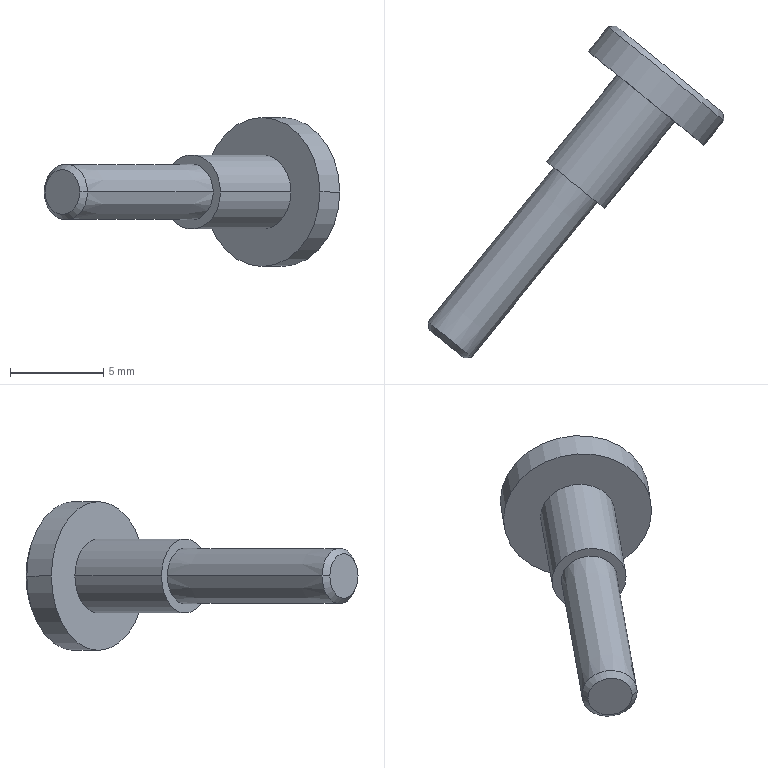Part | SolidWorks | features BaseBody 1 | 1 solid | 14 faces | box 15.875 x 17.831 x 8 mm | volume 252.086 mm3 | cone 6 | cylinder 4 | plane 4 | commonest cylinder face diameters 4 x2 8 x2
STEP:
#1=CARTESIAN_POINT('',(502.793,-146.387,330.545));
#2=VERTEX_POINT('',#1);
#3=CARTESIAN_POINT('',(505.117,-148.278,330.545));
#4=VERTEX_POINT('',#3);
#5=CARTESIAN_POINT('',(503.955,-147.333,330.545));
#6=DIRECTION('',(0.6309,0.7758,-0.000000012));
#7=DIRECTION('',(-0.4361,0.3546,-0.8271));
#8=AXIS2_PLACEMENT_3D('',#5,#6,#7);
#9=CIRCLE('',#8,1.498);
#10=EDGE_CURVE('',#2,#4,#9,.T.);
#11=ORIENTED_EDGE('',*,*,#10,.T.);
#12=CARTESIAN_POINT('',(511.87,-139.977,330.545));
#13=VERTEX_POINT('',#12);
#14=CARTESIAN_POINT('',(511.87,-139.977,330.545));
#15=DIRECTION('',(0.6311,0.7757,-0.000000012));
#16=VECTOR('',#15,1000.);
#17=LINE('',#14,#16);
#18=EDGE_CURVE('',#4,#13,#17,.T.);
#19=ORIENTED_EDGE('',*,*,#18,.T.);
#20=CARTESIAN_POINT('',(509.542,-138.085,330.545));
#21=VERTEX_POINT('',#20);
#22=CARTESIAN_POINT('',(510.706,-139.031,330.545));
#23=DIRECTION('',(-0.6309,-0.7758,0.000000012));
#24=DIRECTION('',(-0.7758,0.6309,0.));
#25=AXIS2_PLACEMENT_3D('',#22,#23,#24);
#26=CIRCLE('',#25,1.5);
#27=EDGE_CURVE('',#13,#21,#26,.T.);
#28=ORIENTED_EDGE('',*,*,#27,.T.);
#29=CARTESIAN_POINT('',(509.542,-138.085,330.545));
#30=DIRECTION('',(0.6308,0.7759,-0.000000012));
#31=VECTOR('',#30,1000.);
#32=LINE('',#29,#31);
#33=EDGE_CURVE('',#2,#21,#32,.T.);
#34=ORIENTED_EDGE('',*,*,#33,.F.);
#35=EDGE_LOOP('',(#11,#19,#28,#34));
#36=FACE_OUTER_BOUND('',#35,.T.);
#37=CARTESIAN_POINT('',(510.706,-139.031,330.545));
#38=DIRECTION('',(0.6309,0.7758,-0.000000012));
#39=DIRECTION('',(-0.7758,0.6309,0.));
#40=AXIS2_PLACEMENT_3D('',#37,#38,#39);
#41=CONICAL_SURFACE('',#40,1.5,0.0001745);
#42=ADVANCED_FACE('',(#36),#41,.T.);
#43=CARTESIAN_POINT('',(502.836,-146.809,330.545));
#44=VERTEX_POINT('',#43);
#45=CARTESIAN_POINT('',(504.695,-148.321,330.545));
#46=VERTEX_POINT('',#45);
#47=CARTESIAN_POINT('',(503.766,-147.565,330.545));
#48=DIRECTION('',(0.6309,0.7758,-0.000000012));
#49=DIRECTION('',(-0.7758,0.6309,0.));
#50=AXIS2_PLACEMENT_3D('',#47,#48,#49);
#51=CIRCLE('',#50,1.198);
#52=EDGE_CURVE('',#44,#46,#51,.T.);
#53=ORIENTED_EDGE('',*,*,#52,.T.);
#54=CARTESIAN_POINT('',(505.117,-148.278,330.545));
#55=DIRECTION('',(0.9947,0.1024,-0.000000009));
#56=VECTOR('',#55,1000.);
#57=LINE('',#54,#56);
#58=EDGE_CURVE('',#46,#4,#57,.T.);
#59=ORIENTED_EDGE('',*,*,#58,.T.);
#60=ORIENTED_EDGE('',*,*,#10,.F.);
#61=CARTESIAN_POINT('',(502.793,-146.387,330.545));
#62=DIRECTION('',(-0.1026,0.9947,-0.000000009));
#63=VECTOR('',#62,1000.);
#64=LINE('',#61,#63);
#65=EDGE_CURVE('',#44,#2,#64,.T.);
#66=ORIENTED_EDGE('',*,*,#65,.F.);
#67=EDGE_LOOP('',(#53,#59,#60,#66));
#68=FACE_OUTER_BOUND('',#67,.T.);
#69=CARTESIAN_POINT('',(503.955,-147.333,330.545));
#70=DIRECTION('',(0.6309,0.7758,-0.000000012));
#71=DIRECTION('',(-0.7758,0.6309,0.));
#72=AXIS2_PLACEMENT_3D('',#69,#70,#71);
#73=CONICAL_SURFACE('',#72,1.498,0.7855);
#74=ADVANCED_FACE('',(#68),#73,.T.);
#75=CARTESIAN_POINT('',(512.258,-140.293,330.545));
#76=VERTEX_POINT('',#75);
#77=CARTESIAN_POINT('',(509.154,-137.769,330.545));
#78=VERTEX_POINT('',#77);
#79=CARTESIAN_POINT('',(510.706,-139.031,330.545));
#80=DIRECTION('',(-0.6309,-0.7758,0.000000012));
#81=DIRECTION('',(-0.7758,0.6309,0.));
#82=AXIS2_PLACEMENT_3D('',#79,#80,#81);
#83=CIRCLE('',#82,2.);
#84=EDGE_CURVE('',#76,#78,#83,.T.);
#85=ORIENTED_EDGE('',*,*,#84,.F.);
#86=CARTESIAN_POINT('',(516.043,-135.638,330.545));
#87=VERTEX_POINT('',#86);
#88=CARTESIAN_POINT('',(516.043,-135.638,330.545));
#89=DIRECTION('',(0.6309,0.7758,-0.000000012));
#90=VECTOR('',#89,1000.);
#91=LINE('',#88,#90);
#92=EDGE_CURVE('',#76,#87,#91,.T.);
#93=ORIENTED_EDGE('',*,*,#92,.T.);
#94=CARTESIAN_POINT('',(512.94,-133.114,330.545));
#95=VERTEX_POINT('',#94);
#96=CARTESIAN_POINT('',(514.492,-134.376,330.545));
#97=DIRECTION('',(-0.6309,-0.7758,0.000000012));
#98=DIRECTION('',(-0.7758,0.6309,0.));
#99=AXIS2_PLACEMENT_3D('',#96,#97,#98);
#100=CIRCLE('',#99,2.);
#101=EDGE_CURVE('',#87,#95,#100,.T.);
#102=ORIENTED_EDGE('',*,*,#101,.T.);
#103=CARTESIAN_POINT('',(512.94,-133.114,330.545));
#104=DIRECTION('',(0.6309,0.7758,-0.000000012));
#105=VECTOR('',#104,1000.);
#106=LINE('',#103,#105);
#107=EDGE_CURVE('',#78,#95,#106,.T.);
#108=ORIENTED_EDGE('',*,*,#107,.F.);
#109=EDGE_LOOP('',(#85,#93,#102,#108));
#110=FACE_OUTER_BOUND('',#109,.T.);
#111=CARTESIAN_POINT('',(514.492,-134.376,330.545));
#112=DIRECTION('',(0.6309,0.7758,-0.000000012));
#113=DIRECTION('',(-0.7758,0.6309,0.));
#114=AXIS2_PLACEMENT_3D('',#111,#112,#113);
#115=CYLINDRICAL_SURFACE('',#114,2.);
#116=ADVANCED_FACE('',(#110),#115,.T.);
#117=CARTESIAN_POINT('',(517.595,-136.9,330.545));
#118=VERTEX_POINT('',#117);
#119=CARTESIAN_POINT('',(511.388,-131.852,330.545));
#120=VERTEX_POINT('',#119);
#121=CARTESIAN_POINT('',(514.492,-134.376,330.545));
#122=DIRECTION('',(-0.6309,-0.7758,0.000000012));
#123=DIRECTION('',(-0.7758,0.6309,0.));
#124=AXIS2_PLACEMENT_3D('',#121,#122,#123);
#125=CIRCLE('',#124,4.);
#126=EDGE_CURVE('',#118,#120,#125,.T.);
#127=ORIENTED_EDGE('',*,*,#126,.F.);
#128=CARTESIAN_POINT('',(518.668,-135.581,330.545));
#129=VERTEX_POINT('',#128);
#130=CARTESIAN_POINT('',(518.857,-135.348,330.545));
#131=DIRECTION('',(0.6309,0.7758,-0.000000012));
#132=VECTOR('',#131,1000.);
#133=LINE('',#130,#132);
#134=EDGE_CURVE('',#118,#129,#133,.T.);
#135=ORIENTED_EDGE('',*,*,#134,.T.);
#136=CARTESIAN_POINT('',(512.461,-130.533,330.545));
#137=VERTEX_POINT('',#136);
#138=CARTESIAN_POINT('',(515.564,-133.057,330.545));
#139=DIRECTION('',(-0.6309,-0.7758,0.000000012));
#140=DIRECTION('',(-0.7758,0.6309,0.));
#141=AXIS2_PLACEMENT_3D('',#138,#139,#140);
#142=CIRCLE('',#141,4.);
#143=EDGE_CURVE('',#129,#137,#142,.T.);
#144=ORIENTED_EDGE('',*,*,#143,.T.);
#145=CARTESIAN_POINT('',(512.65,-130.301,330.545));
#146=DIRECTION('',(0.6309,0.7758,-0.000000012));
#147=VECTOR('',#146,1000.);
#148=LINE('',#145,#147);
#149=EDGE_CURVE('',#120,#137,#148,.T.);
#150=ORIENTED_EDGE('',*,*,#149,.F.);
#151=EDGE_LOOP('',(#127,#135,#144,#150));
#152=FACE_OUTER_BOUND('',#151,.T.);
#153=CARTESIAN_POINT('',(515.753,-132.824,330.545));
#154=DIRECTION('',(0.6309,0.7758,-0.000000012));
#155=DIRECTION('',(-0.7758,0.6309,0.));
#156=AXIS2_PLACEMENT_3D('',#153,#154,#155);
#157=CYLINDRICAL_SURFACE('',#156,4.);
#158=ADVANCED_FACE('',(#152),#157,.T.);
#159=CARTESIAN_POINT('',(518.624,-135.159,330.545));
#160=VERTEX_POINT('',#159);
#161=CARTESIAN_POINT('',(512.883,-130.49,330.545));
#162=VERTEX_POINT('',#161);
#163=CARTESIAN_POINT('',(515.753,-132.824,330.545));
#164=DIRECTION('',(-0.6309,-0.7758,0.000000012));
#165=DIRECTION('',(0.7758,-0.6309,0.));
#166=AXIS2_PLACEMENT_3D('',#163,#164,#165);
#167=CIRCLE('',#166,3.7);
#168=EDGE_CURVE('',#160,#162,#167,.T.);
#169=ORIENTED_EDGE('',*,*,#168,.T.);
#170=CARTESIAN_POINT('',(512.461,-130.533,330.545));
#171=DIRECTION('',(-0.9947,-0.1025,0.000000009));
#172=VECTOR('',#171,1000.);
#173=LINE('',#170,#172);
#174=EDGE_CURVE('',#162,#137,#173,.T.);
#175=ORIENTED_EDGE('',*,*,#174,.T.);
#176=ORIENTED_EDGE('',*,*,#143,.F.);
#177=CARTESIAN_POINT('',(518.668,-135.581,330.545));
#178=DIRECTION('',(0.1025,-0.9947,0.000000009));
#179=VECTOR('',#178,1000.);
#180=LINE('',#177,#179);
#181=EDGE_CURVE('',#160,#129,#180,.T.);
#182=ORIENTED_EDGE('',*,*,#181,.F.);
#183=EDGE_LOOP('',(#169,#175,#176,#182));
#184=FACE_OUTER_BOUND('',#183,.T.);
#185=CARTESIAN_POINT('',(515.564,-133.057,330.545));
#186=DIRECTION('',(-0.6309,-0.7758,0.000000012));
#187=DIRECTION('',(0.7758,-0.6309,0.));
#188=AXIS2_PLACEMENT_3D('',#185,#186,#187);
#189=CONICAL_SURFACE('',#188,4.,0.7854);
#190=ADVANCED_FACE('',(#184),#189,.T.);
#191=ORIENTED_EDGE('',*,*,#18,.F.);
#192=CARTESIAN_POINT('',(503.955,-147.333,330.545));
#193=DIRECTION('',(0.6309,0.7758,-0.000000012));
#194=DIRECTION('',(-0.4361,0.3546,-0.8271));
#195=AXIS2_PLACEMENT_3D('',#192,#193,#194);
#196=CIRCLE('',#195,1.498);
#197=EDGE_CURVE('',#4,#2,#196,.T.);
#198=ORIENTED_EDGE('',*,*,#197,.T.);
#199=ORIENTED_EDGE('',*,*,#33,.T.);
#200=CARTESIAN_POINT('',(510.706,-139.031,330.545));
#201=DIRECTION('',(-0.6309,-0.7758,0.000000012));
#202=DIRECTION('',(-0.7758,0.6309,0.));
#203=AXIS2_PLACEMENT_3D('',#200,#201,#202);
#204=CIRCLE('',#203,1.5);
#205=EDGE_CURVE('',#21,#13,#204,.T.);
#206=ORIENTED_EDGE('',*,*,#205,.T.);
#207=EDGE_LOOP('',(#191,#198,#199,#206));
#208=FACE_OUTER_BOUND('',#207,.T.);
#209=CARTESIAN_POINT('',(510.706,-139.031,330.545));
#210=DIRECTION('',(0.6309,0.7758,-0.000000012));
#211=DIRECTION('',(-0.7758,0.6309,0.));
#212=AXIS2_PLACEMENT_3D('',#209,#210,#211);
#213=CONICAL_SURFACE('',#212,1.5,0.0001745);
#214=ADVANCED_FACE('',(#208),#213,.T.);
#215=CARTESIAN_POINT('',(510.706,-139.031,330.545));
#216=DIRECTION('',(-0.6309,-0.7758,0.000000012));
#217=DIRECTION('',(-0.7758,0.6309,0.));
#218=AXIS2_PLACEMENT_3D('',#215,#216,#217);
#219=CIRCLE('',#218,2.);
#220=EDGE_CURVE('',#78,#76,#219,.T.);
#221=ORIENTED_EDGE('',*,*,#220,.T.);
#222=ORIENTED_EDGE('',*,*,#84,.T.);
#223=EDGE_LOOP('',(#221,#222));
#224=FACE_OUTER_BOUND('',#223,.T.);
#225=ORIENTED_EDGE('',*,*,#205,.F.);
#226=ORIENTED_EDGE('',*,*,#27,.F.);
#227=EDGE_LOOP('',(#225,#226));
#228=FACE_BOUND('',#227,.T.);
#229=CARTESIAN_POINT('',(510.706,-139.031,330.545));
#230=DIRECTION('',(-0.6309,-0.7758,0.000000012));
#231=DIRECTION('',(0.7758,-0.6309,0.));
#232=AXIS2_PLACEMENT_3D('',#229,#230,#231);
#233=PLANE('',#232);
#234=ADVANCED_FACE('',(#224,#228),#233,.T.);
#235=ORIENTED_EDGE('',*,*,#58,.F.);
#236=CARTESIAN_POINT('',(503.766,-147.565,330.545));
#237=DIRECTION('',(0.6309,0.7758,-0.000000012));
#238=DIRECTION('',(-0.7758,0.6309,0.));
#239=AXIS2_PLACEMENT_3D('',#236,#237,#238);
#240=CIRCLE('',#239,1.198);
#241=EDGE_CURVE('',#46,#44,#240,.T.);
#242=ORIENTED_EDGE('',*,*,#241,.T.);
#243=ORIENTED_EDGE('',*,*,#65,.T.);
#244=ORIENTED_EDGE('',*,*,#197,.F.);
#245=EDGE_LOOP('',(#235,#242,#243,#244));
#246=FACE_OUTER_BOUND('',#245,.T.);
#247=CARTESIAN_POINT('',(503.955,-147.333,330.545));
#248=DIRECTION('',(0.6309,0.7758,-0.000000012));
#249=DIRECTION('',(-0.7758,0.6309,0.));
#250=AXIS2_PLACEMENT_3D('',#247,#248,#249);
#251=CONICAL_SURFACE('',#250,1.498,0.7855);
#252=ADVANCED_FACE('',(#246),#251,.T.);
#253=ORIENTED_EDGE('',*,*,#92,.F.);
#254=ORIENTED_EDGE('',*,*,#220,.F.);
#255=ORIENTED_EDGE('',*,*,#107,.T.);
#256=CARTESIAN_POINT('',(514.492,-134.376,330.545));
#257=DIRECTION('',(-0.6309,-0.7758,0.000000012));
#258=DIRECTION('',(-0.7758,0.6309,0.));
#259=AXIS2_PLACEMENT_3D('',#256,#257,#258);
#260=CIRCLE('',#259,2.);
#261=EDGE_CURVE('',#95,#87,#260,.T.);
#262=ORIENTED_EDGE('',*,*,#261,.T.);
#263=EDGE_LOOP('',(#253,#254,#255,#262));
#264=FACE_OUTER_BOUND('',#263,.T.);
#265=CARTESIAN_POINT('',(514.492,-134.376,330.545));
#266=DIRECTION('',(0.6309,0.7758,-0.000000012));
#267=DIRECTION('',(-0.7758,0.6309,0.));
#268=AXIS2_PLACEMENT_3D('',#265,#266,#267);
#269=CYLINDRICAL_SURFACE('',#268,2.);
#270=ADVANCED_FACE('',(#264),#269,.T.);
#271=ORIENTED_EDGE('',*,*,#52,.F.);
#272=ORIENTED_EDGE('',*,*,#241,.F.);
#273=EDGE_LOOP('',(#271,#272));
#274=FACE_OUTER_BOUND('',#273,.T.);
#275=CARTESIAN_POINT('',(503.766,-147.565,330.545));
#276=DIRECTION('',(-0.6309,-0.7758,0.000000012));
#277=DIRECTION('',(0.7758,-0.6309,0.));
#278=AXIS2_PLACEMENT_3D('',#275,#276,#277);
#279=PLANE('',#278);
#280=ADVANCED_FACE('',(#274),#279,.T.);
#281=CARTESIAN_POINT('',(514.492,-134.376,330.545));
#282=DIRECTION('',(-0.6309,-0.7758,0.000000012));
#283=DIRECTION('',(-0.7758,0.6309,0.));
#284=AXIS2_PLACEMENT_3D('',#281,#282,#283);
#285=CIRCLE('',#284,4.);
#286=EDGE_CURVE('',#120,#118,#285,.T.);
#287=ORIENTED_EDGE('',*,*,#286,.T.);
#288=ORIENTED_EDGE('',*,*,#126,.T.);
#289=EDGE_LOOP('',(#287,#288));
#290=FACE_OUTER_BOUND('',#289,.T.);
#291=ORIENTED_EDGE('',*,*,#261,.F.);
#292=ORIENTED_EDGE('',*,*,#101,.F.);
#293=EDGE_LOOP('',(#291,#292));
#294=FACE_BOUND('',#293,.T.);
#295=CARTESIAN_POINT('',(514.492,-134.376,330.545));
#296=DIRECTION('',(-0.6309,-0.7758,0.000000012));
#297=DIRECTION('',(0.7758,-0.6309,0.));
#298=AXIS2_PLACEMENT_3D('',#295,#296,#297);
#299=PLANE('',#298);
#300=ADVANCED_FACE('',(#290,#294),#299,.T.);
#301=ORIENTED_EDGE('',*,*,#134,.F.);
#302=ORIENTED_EDGE('',*,*,#286,.F.);
#303=ORIENTED_EDGE('',*,*,#149,.T.);
#304=CARTESIAN_POINT('',(515.564,-133.057,330.545));
#305=DIRECTION('',(-0.6309,-0.7758,0.000000012));
#306=DIRECTION('',(-0.7758,0.6309,0.));
#307=AXIS2_PLACEMENT_3D('',#304,#305,#306);
#308=CIRCLE('',#307,4.);
#309=EDGE_CURVE('',#137,#129,#308,.T.);
#310=ORIENTED_EDGE('',*,*,#309,.T.);
#311=EDGE_LOOP('',(#301,#302,#303,#310));
#312=FACE_OUTER_BOUND('',#311,.T.);
#313=CARTESIAN_POINT('',(515.753,-132.824,330.545));
#314=DIRECTION('',(0.6309,0.7758,-0.000000012));
#315=DIRECTION('',(-0.7758,0.6309,0.));
#316=AXIS2_PLACEMENT_3D('',#313,#314,#315);
#317=CYLINDRICAL_SURFACE('',#316,4.);
#318=ADVANCED_FACE('',(#312),#317,.T.);
#319=ORIENTED_EDGE('',*,*,#174,.F.);
#320=CARTESIAN_POINT('',(515.753,-132.824,330.545));
#321=DIRECTION('',(-0.6309,-0.7758,0.000000012));
#322=DIRECTION('',(0.7758,-0.6309,0.));
#323=AXIS2_PLACEMENT_3D('',#320,#321,#322);
#324=CIRCLE('',#323,3.7);
#325=EDGE_CURVE('',#162,#160,#324,.T.);
#326=ORIENTED_EDGE('',*,*,#325,.T.);
#327=ORIENTED_EDGE('',*,*,#181,.T.);
#328=ORIENTED_EDGE('',*,*,#309,.F.);
#329=EDGE_LOOP('',(#319,#326,#327,#328));
#330=FACE_OUTER_BOUND('',#329,.T.);
#331=CARTESIAN_POINT('',(515.564,-133.057,330.545));
#332=DIRECTION('',(-0.6309,-0.7758,0.000000012));
#333=DIRECTION('',(0.7758,-0.6309,0.));
#334=AXIS2_PLACEMENT_3D('',#331,#332,#333);
#335=CONICAL_SURFACE('',#334,4.,0.7854);
#336=ADVANCED_FACE('',(#330),#335,.T.);
#337=ORIENTED_EDGE('',*,*,#168,.F.);
#338=ORIENTED_EDGE('',*,*,#325,.F.);
#339=EDGE_LOOP('',(#337,#338));
#340=FACE_OUTER_BOUND('',#339,.T.);
#341=CARTESIAN_POINT('',(515.753,-132.824,330.545));
#342=DIRECTION('',(-0.6309,-0.7758,0.000000012));
#343=DIRECTION('',(0.7758,-0.6309,0.));
#344=AXIS2_PLACEMENT_3D('',#341,#342,#343);
#345=PLANE('',#344);
#346=ADVANCED_FACE('',(#340),#345,.F.);
#347=CLOSED_SHELL('',(#42,#74,#116,#158,#190,#214,#234,#252,#270,#280,#300,#318,#336,#346));
#348=MANIFOLD_SOLID_BREP('',#347);
#349=CARTESIAN_POINT('',(0.,0.,0.));
#350=DIRECTION('',(0.,0.,1.));
#351=DIRECTION('',(1.,0.,0.));
#352=AXIS2_PLACEMENT_3D('',#349,#350,#351);
#353=(LENGTH_UNIT()NAMED_UNIT(*)SI_UNIT(.MILLI.,.METRE.));
#354=UNCERTAINTY_MEASURE_WITH_UNIT(LENGTH_MEASURE(0.00001),#353,'','');
#355=(NAMED_UNIT(*)PLANE_ANGLE_UNIT()SI_UNIT($,.RADIAN.));
#356=(NAMED_UNIT(*)SI_UNIT($,.STERADIAN.)SOLID_ANGLE_UNIT());
#357=(GEOMETRIC_REPRESENTATION_CONTEXT(3)GLOBAL_UNCERTAINTY_ASSIGNED_CONTEXT((#354))GLOBAL_UNIT_ASSIGNED_CONTEXT((#353,#355,#356))REPRESENTATION_CONTEXT('',''));
#358=ADVANCED_BREP_SHAPE_REPRESENTATION('',(#348,#352),#357);